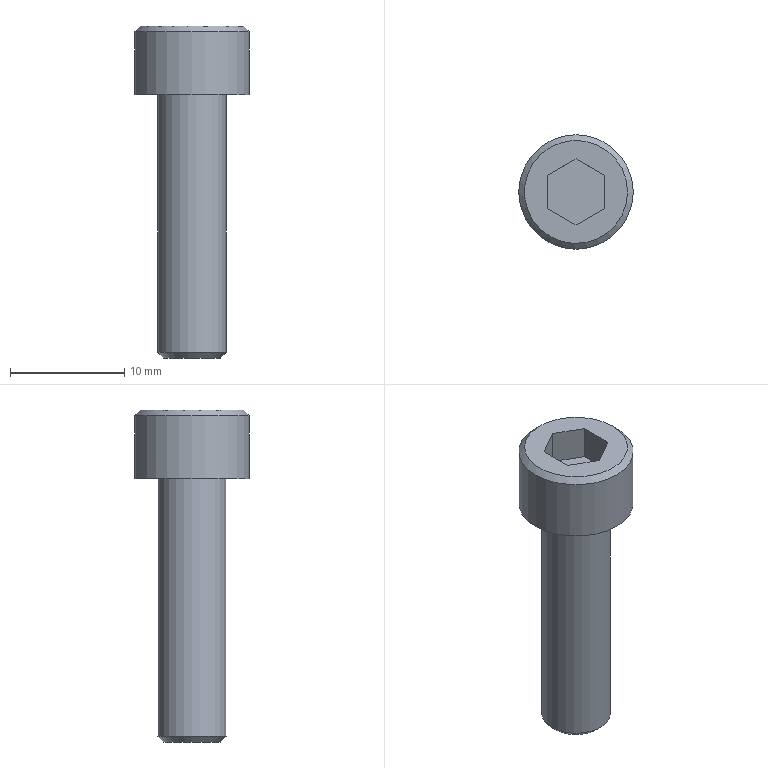Part | STEP file | M6.00-20.00_id118_x_t | 1 solid | 14 faces | box 10 x 10 x 29 mm | volume 1051 mm3 | plane 10 | cylinder 2 | cone 2 | commonest cylinder face diameters 6 x1 10 x1
STEP:
#1=CARTESIAN_POINT('',(-35.5,-80.,-101.5));
#2=VERTEX_POINT('',#1);
#3=CARTESIAN_POINT('',(-40.,-80.,-101.5));
#4=DIRECTION('',(0.,0.,1.));
#5=DIRECTION('',(1.,0.,0.));
#6=AXIS2_PLACEMENT_3D('',#3,#4,#5);
#7=CIRCLE('',#6,4.5);
#8=EDGE_CURVE('',#2,#2,#7,.T.);
#9=ORIENTED_EDGE('',*,*,#8,.T.);
#10=EDGE_LOOP('',(#9));
#11=FACE_BOUND('',#10,.T.);
#12=CARTESIAN_POINT('',(-42.5,-78.557,-101.5));
#13=VERTEX_POINT('',#12);
#14=CARTESIAN_POINT('',(-42.5,-81.443,-101.5));
#15=VERTEX_POINT('',#14);
#16=CARTESIAN_POINT('',(-42.5,-78.557,-101.5));
#17=DIRECTION('',(0.,-1.,0.));
#18=VECTOR('',#17,1.);
#19=LINE('',#16,#18);
#20=EDGE_CURVE('',#13,#15,#19,.T.);
#21=ORIENTED_EDGE('',*,*,#20,.F.);
#22=CARTESIAN_POINT('',(-40.,-77.113,-101.5));
#23=VERTEX_POINT('',#22);
#24=CARTESIAN_POINT('',(-40.,-77.113,-101.5));
#25=DIRECTION('',(-0.866,-0.5,0.));
#26=VECTOR('',#25,1.);
#27=LINE('',#24,#26);
#28=EDGE_CURVE('',#23,#13,#27,.T.);
#29=ORIENTED_EDGE('',*,*,#28,.F.);
#30=CARTESIAN_POINT('',(-37.5,-78.557,-101.5));
#31=VERTEX_POINT('',#30);
#32=CARTESIAN_POINT('',(-37.5,-78.557,-101.5));
#33=DIRECTION('',(-0.866,0.5,0.));
#34=VECTOR('',#33,1.);
#35=LINE('',#32,#34);
#36=EDGE_CURVE('',#31,#23,#35,.T.);
#37=ORIENTED_EDGE('',*,*,#36,.F.);
#38=CARTESIAN_POINT('',(-37.5,-81.443,-101.5));
#39=VERTEX_POINT('',#38);
#40=CARTESIAN_POINT('',(-37.5,-81.443,-101.5));
#41=DIRECTION('',(0.,1.,0.));
#42=VECTOR('',#41,1.);
#43=LINE('',#40,#42);
#44=EDGE_CURVE('',#39,#31,#43,.T.);
#45=ORIENTED_EDGE('',*,*,#44,.F.);
#46=CARTESIAN_POINT('',(-40.,-82.887,-101.5));
#47=VERTEX_POINT('',#46);
#48=CARTESIAN_POINT('',(-40.,-82.887,-101.5));
#49=DIRECTION('',(0.866,0.5,0.));
#50=VECTOR('',#49,1.);
#51=LINE('',#48,#50);
#52=EDGE_CURVE('',#47,#39,#51,.T.);
#53=ORIENTED_EDGE('',*,*,#52,.F.);
#54=CARTESIAN_POINT('',(-42.5,-81.443,-101.5));
#55=DIRECTION('',(0.866,-0.5,0.));
#56=VECTOR('',#55,1.);
#57=LINE('',#54,#56);
#58=EDGE_CURVE('',#15,#47,#57,.T.);
#59=ORIENTED_EDGE('',*,*,#58,.F.);
#60=EDGE_LOOP('',(#21,#29,#37,#45,#53,#59));
#61=FACE_BOUND('',#60,.T.);
#62=CARTESIAN_POINT('',(-40.,-80.,-101.5));
#63=DIRECTION('',(0.,0.,1.));
#64=DIRECTION('',(1.,0.,0.));
#65=AXIS2_PLACEMENT_3D('',#62,#63,#64);
#66=PLANE('',#65);
#67=ADVANCED_FACE('',(#11,#61),#66,.T.);
#68=CARTESIAN_POINT('',(-43.,-80.,-107.5));
#69=VERTEX_POINT('',#68);
#70=CARTESIAN_POINT('',(-40.,-80.,-107.5));
#71=DIRECTION('',(0.,0.,-1.));
#72=DIRECTION('',(-1.,0.,0.));
#73=AXIS2_PLACEMENT_3D('',#70,#71,#72);
#74=CIRCLE('',#73,3.);
#75=EDGE_CURVE('',#69,#69,#74,.T.);
#76=ORIENTED_EDGE('',*,*,#75,.F.);
#77=EDGE_LOOP('',(#76));
#78=FACE_BOUND('',#77,.T.);
#79=CARTESIAN_POINT('',(-35.,-80.,-107.5));
#80=VERTEX_POINT('',#79);
#81=CARTESIAN_POINT('',(-40.,-80.,-107.5));
#82=DIRECTION('',(0.,0.,1.));
#83=DIRECTION('',(1.,0.,0.));
#84=AXIS2_PLACEMENT_3D('',#81,#82,#83);
#85=CIRCLE('',#84,5.);
#86=EDGE_CURVE('',#80,#80,#85,.T.);
#87=ORIENTED_EDGE('',*,*,#86,.F.);
#88=EDGE_LOOP('',(#87));
#89=FACE_BOUND('',#88,.T.);
#90=CARTESIAN_POINT('',(-40.,-80.,-107.5));
#91=DIRECTION('',(0.,0.,-1.));
#92=DIRECTION('',(-1.,0.,0.));
#93=AXIS2_PLACEMENT_3D('',#90,#91,#92);
#94=PLANE('',#93);
#95=ADVANCED_FACE('',(#78,#89),#94,.T.);
#96=CARTESIAN_POINT('',(-35.,-80.,-102.));
#97=VERTEX_POINT('',#96);
#98=CARTESIAN_POINT('',(-40.,-80.,-102.));
#99=DIRECTION('',(0.,0.,-1.));
#100=DIRECTION('',(1.,0.,0.));
#101=AXIS2_PLACEMENT_3D('',#98,#99,#100);
#102=CIRCLE('',#101,5.);
#103=EDGE_CURVE('',#97,#97,#102,.T.);
#104=ORIENTED_EDGE('',*,*,#103,.T.);
#105=EDGE_LOOP('',(#104));
#106=FACE_BOUND('',#105,.T.);
#107=ORIENTED_EDGE('',*,*,#86,.T.);
#108=EDGE_LOOP('',(#107));
#109=FACE_BOUND('',#108,.T.);
#110=CARTESIAN_POINT('',(-40.,-80.,-107.5));
#111=DIRECTION('',(0.,0.,1.));
#112=DIRECTION('',(1.,0.,0.));
#113=AXIS2_PLACEMENT_3D('',#110,#111,#112);
#114=CYLINDRICAL_SURFACE('',#113,5.);
#115=ADVANCED_FACE('',(#106,#109),#114,.T.);
#116=CARTESIAN_POINT('',(-42.5,-80.,-130.5));
#117=VERTEX_POINT('',#116);
#118=CARTESIAN_POINT('',(-40.,-80.,-130.5));
#119=DIRECTION('',(0.,0.,-1.));
#120=DIRECTION('',(-1.,0.,0.));
#121=AXIS2_PLACEMENT_3D('',#118,#119,#120);
#122=CIRCLE('',#121,2.5);
#123=EDGE_CURVE('',#117,#117,#122,.T.);
#124=ORIENTED_EDGE('',*,*,#123,.T.);
#125=EDGE_LOOP('',(#124));
#126=FACE_OUTER_BOUND('',#125,.T.);
#127=CARTESIAN_POINT('',(-40.,-80.,-130.5));
#128=DIRECTION('',(0.,0.,-1.));
#129=DIRECTION('',(-1.,0.,0.));
#130=AXIS2_PLACEMENT_3D('',#127,#128,#129);
#131=PLANE('',#130);
#132=ADVANCED_FACE('',(#126),#131,.T.);
#133=CARTESIAN_POINT('',(-43.,-80.,-130.));
#134=VERTEX_POINT('',#133);
#135=CARTESIAN_POINT('',(-40.,-80.,-130.));
#136=DIRECTION('',(0.,0.,1.));
#137=DIRECTION('',(-1.,0.,0.));
#138=AXIS2_PLACEMENT_3D('',#135,#136,#137);
#139=CIRCLE('',#138,3.);
#140=EDGE_CURVE('',#134,#134,#139,.T.);
#141=ORIENTED_EDGE('',*,*,#140,.T.);
#142=EDGE_LOOP('',(#141));
#143=FACE_BOUND('',#142,.T.);
#144=ORIENTED_EDGE('',*,*,#75,.T.);
#145=EDGE_LOOP('',(#144));
#146=FACE_BOUND('',#145,.T.);
#147=CARTESIAN_POINT('',(-40.,-80.,-107.5));
#148=DIRECTION('',(0.,0.,-1.));
#149=DIRECTION('',(-1.,0.,0.));
#150=AXIS2_PLACEMENT_3D('',#147,#148,#149);
#151=CYLINDRICAL_SURFACE('',#150,3.);
#152=ADVANCED_FACE('',(#143,#146),#151,.T.);
#153=ORIENTED_EDGE('',*,*,#58,.T.);
#154=CARTESIAN_POINT('',(-40.,-82.887,-104.5));
#155=VERTEX_POINT('',#154);
#156=CARTESIAN_POINT('',(-40.,-82.887,-104.5));
#157=DIRECTION('',(0.,0.,1.));
#158=VECTOR('',#157,1.);
#159=LINE('',#156,#158);
#160=EDGE_CURVE('',#155,#47,#159,.T.);
#161=ORIENTED_EDGE('',*,*,#160,.F.);
#162=CARTESIAN_POINT('',(-42.5,-81.443,-104.5));
#163=VERTEX_POINT('',#162);
#164=CARTESIAN_POINT('',(-42.5,-81.443,-104.5));
#165=DIRECTION('',(0.866,-0.5,0.));
#166=VECTOR('',#165,1.);
#167=LINE('',#164,#166);
#168=EDGE_CURVE('',#163,#155,#167,.T.);
#169=ORIENTED_EDGE('',*,*,#168,.F.);
#170=CARTESIAN_POINT('',(-42.5,-81.443,-104.5));
#171=DIRECTION('',(0.,0.,1.));
#172=VECTOR('',#171,1.);
#173=LINE('',#170,#172);
#174=EDGE_CURVE('',#163,#15,#173,.T.);
#175=ORIENTED_EDGE('',*,*,#174,.T.);
#176=EDGE_LOOP('',(#153,#161,#169,#175));
#177=FACE_OUTER_BOUND('',#176,.T.);
#178=CARTESIAN_POINT('',(-41.25,-82.165,-103.));
#179=DIRECTION('',(-0.5,-0.866,0.));
#180=DIRECTION('',(0.866,-0.5,0.));
#181=AXIS2_PLACEMENT_3D('',#178,#179,#180);
#182=PLANE('',#181);
#183=ADVANCED_FACE('',(#177),#182,.F.);
#184=ORIENTED_EDGE('',*,*,#20,.T.);
#185=ORIENTED_EDGE('',*,*,#174,.F.);
#186=CARTESIAN_POINT('',(-42.5,-78.557,-104.5));
#187=VERTEX_POINT('',#186);
#188=CARTESIAN_POINT('',(-42.5,-78.557,-104.5));
#189=DIRECTION('',(0.,-1.,0.));
#190=VECTOR('',#189,1.);
#191=LINE('',#188,#190);
#192=EDGE_CURVE('',#187,#163,#191,.T.);
#193=ORIENTED_EDGE('',*,*,#192,.F.);
#194=CARTESIAN_POINT('',(-42.5,-78.557,-104.5));
#195=DIRECTION('',(0.,0.,1.));
#196=VECTOR('',#195,1.);
#197=LINE('',#194,#196);
#198=EDGE_CURVE('',#187,#13,#197,.T.);
#199=ORIENTED_EDGE('',*,*,#198,.T.);
#200=EDGE_LOOP('',(#184,#185,#193,#199));
#201=FACE_OUTER_BOUND('',#200,.T.);
#202=CARTESIAN_POINT('',(-42.5,-80.,-103.));
#203=DIRECTION('',(-1.,0.,0.));
#204=DIRECTION('',(0.,0.,1.));
#205=AXIS2_PLACEMENT_3D('',#202,#203,#204);
#206=PLANE('',#205);
#207=ADVANCED_FACE('',(#201),#206,.F.);
#208=ORIENTED_EDGE('',*,*,#28,.T.);
#209=ORIENTED_EDGE('',*,*,#198,.F.);
#210=CARTESIAN_POINT('',(-40.,-77.113,-104.5));
#211=VERTEX_POINT('',#210);
#212=CARTESIAN_POINT('',(-40.,-77.113,-104.5));
#213=DIRECTION('',(-0.866,-0.5,0.));
#214=VECTOR('',#213,1.);
#215=LINE('',#212,#214);
#216=EDGE_CURVE('',#211,#187,#215,.T.);
#217=ORIENTED_EDGE('',*,*,#216,.F.);
#218=CARTESIAN_POINT('',(-40.,-77.113,-104.5));
#219=DIRECTION('',(0.,0.,1.));
#220=VECTOR('',#219,1.);
#221=LINE('',#218,#220);
#222=EDGE_CURVE('',#211,#23,#221,.T.);
#223=ORIENTED_EDGE('',*,*,#222,.T.);
#224=EDGE_LOOP('',(#208,#209,#217,#223));
#225=FACE_OUTER_BOUND('',#224,.T.);
#226=CARTESIAN_POINT('',(-41.25,-77.835,-103.));
#227=DIRECTION('',(-0.5,0.866,0.));
#228=DIRECTION('',(-0.866,-0.5,0.));
#229=AXIS2_PLACEMENT_3D('',#226,#227,#228);
#230=PLANE('',#229);
#231=ADVANCED_FACE('',(#225),#230,.F.);
#232=ORIENTED_EDGE('',*,*,#36,.T.);
#233=ORIENTED_EDGE('',*,*,#222,.F.);
#234=CARTESIAN_POINT('',(-37.5,-78.557,-104.5));
#235=VERTEX_POINT('',#234);
#236=CARTESIAN_POINT('',(-37.5,-78.557,-104.5));
#237=DIRECTION('',(-0.866,0.5,0.));
#238=VECTOR('',#237,1.);
#239=LINE('',#236,#238);
#240=EDGE_CURVE('',#235,#211,#239,.T.);
#241=ORIENTED_EDGE('',*,*,#240,.F.);
#242=CARTESIAN_POINT('',(-37.5,-78.557,-104.5));
#243=DIRECTION('',(0.,0.,1.));
#244=VECTOR('',#243,1.);
#245=LINE('',#242,#244);
#246=EDGE_CURVE('',#235,#31,#245,.T.);
#247=ORIENTED_EDGE('',*,*,#246,.T.);
#248=EDGE_LOOP('',(#232,#233,#241,#247));
#249=FACE_OUTER_BOUND('',#248,.T.);
#250=CARTESIAN_POINT('',(-38.75,-77.835,-103.));
#251=DIRECTION('',(0.5,0.866,0.));
#252=DIRECTION('',(-0.866,0.5,0.));
#253=AXIS2_PLACEMENT_3D('',#250,#251,#252);
#254=PLANE('',#253);
#255=ADVANCED_FACE('',(#249),#254,.F.);
#256=ORIENTED_EDGE('',*,*,#44,.T.);
#257=ORIENTED_EDGE('',*,*,#246,.F.);
#258=CARTESIAN_POINT('',(-37.5,-81.443,-104.5));
#259=VERTEX_POINT('',#258);
#260=CARTESIAN_POINT('',(-37.5,-81.443,-104.5));
#261=DIRECTION('',(0.,1.,0.));
#262=VECTOR('',#261,1.);
#263=LINE('',#260,#262);
#264=EDGE_CURVE('',#259,#235,#263,.T.);
#265=ORIENTED_EDGE('',*,*,#264,.F.);
#266=CARTESIAN_POINT('',(-37.5,-81.443,-104.5));
#267=DIRECTION('',(0.,0.,1.));
#268=VECTOR('',#267,1.);
#269=LINE('',#266,#268);
#270=EDGE_CURVE('',#259,#39,#269,.T.);
#271=ORIENTED_EDGE('',*,*,#270,.T.);
#272=EDGE_LOOP('',(#256,#257,#265,#271));
#273=FACE_OUTER_BOUND('',#272,.T.);
#274=CARTESIAN_POINT('',(-37.5,-80.,-103.));
#275=DIRECTION('',(1.,0.,0.));
#276=DIRECTION('',(0.,0.,-1.));
#277=AXIS2_PLACEMENT_3D('',#274,#275,#276);
#278=PLANE('',#277);
#279=ADVANCED_FACE('',(#273),#278,.F.);
#280=ORIENTED_EDGE('',*,*,#52,.T.);
#281=ORIENTED_EDGE('',*,*,#270,.F.);
#282=CARTESIAN_POINT('',(-40.,-82.887,-104.5));
#283=DIRECTION('',(0.866,0.5,0.));
#284=VECTOR('',#283,1.);
#285=LINE('',#282,#284);
#286=EDGE_CURVE('',#155,#259,#285,.T.);
#287=ORIENTED_EDGE('',*,*,#286,.F.);
#288=ORIENTED_EDGE('',*,*,#160,.T.);
#289=EDGE_LOOP('',(#280,#281,#287,#288));
#290=FACE_OUTER_BOUND('',#289,.T.);
#291=CARTESIAN_POINT('',(-38.75,-82.165,-103.));
#292=DIRECTION('',(0.5,-0.866,0.));
#293=DIRECTION('',(0.866,0.5,0.));
#294=AXIS2_PLACEMENT_3D('',#291,#292,#293);
#295=PLANE('',#294);
#296=ADVANCED_FACE('',(#290),#295,.F.);
#297=ORIENTED_EDGE('',*,*,#286,.T.);
#298=ORIENTED_EDGE('',*,*,#264,.T.);
#299=ORIENTED_EDGE('',*,*,#240,.T.);
#300=ORIENTED_EDGE('',*,*,#216,.T.);
#301=ORIENTED_EDGE('',*,*,#192,.T.);
#302=ORIENTED_EDGE('',*,*,#168,.T.);
#303=EDGE_LOOP('',(#297,#298,#299,#300,#301,#302));
#304=FACE_OUTER_BOUND('',#303,.T.);
#305=CARTESIAN_POINT('',(-40.,-80.,-104.5));
#306=DIRECTION('',(0.,0.,-1.));
#307=DIRECTION('',(-1.,0.,0.));
#308=AXIS2_PLACEMENT_3D('',#305,#306,#307);
#309=PLANE('',#308);
#310=ADVANCED_FACE('',(#304),#309,.F.);
#311=ORIENTED_EDGE('',*,*,#123,.F.);
#312=EDGE_LOOP('',(#311));
#313=FACE_BOUND('',#312,.T.);
#314=ORIENTED_EDGE('',*,*,#140,.F.);
#315=EDGE_LOOP('',(#314));
#316=FACE_BOUND('',#315,.T.);
#317=CARTESIAN_POINT('',(-40.,-80.,-130.));
#318=DIRECTION('',(0.,0.,1.));
#319=DIRECTION('',(1.,0.,0.));
#320=AXIS2_PLACEMENT_3D('',#317,#318,#319);
#321=CONICAL_SURFACE('',#320,3.,45.);
#322=ADVANCED_FACE('',(#313,#316),#321,.T.);
#323=ORIENTED_EDGE('',*,*,#8,.F.);
#324=EDGE_LOOP('',(#323));
#325=FACE_BOUND('',#324,.T.);
#326=ORIENTED_EDGE('',*,*,#103,.F.);
#327=EDGE_LOOP('',(#326));
#328=FACE_BOUND('',#327,.T.);
#329=CARTESIAN_POINT('',(-40.,-80.,-102.));
#330=DIRECTION('',(0.,0.,-1.));
#331=DIRECTION('',(-1.,0.,0.));
#332=AXIS2_PLACEMENT_3D('',#329,#330,#331);
#333=CONICAL_SURFACE('',#332,5.,45.);
#334=ADVANCED_FACE('',(#325,#328),#333,.T.);
#335=CLOSED_SHELL('',(#67,#95,#115,#132,#152,#183,#207,#231,#255,#279,#296,#310,#322,#334));
#336=MANIFOLD_SOLID_BREP('',#335);
#337=(LENGTH_UNIT()NAMED_UNIT(*)SI_UNIT(.MILLI.,.METRE.));
#338=UNCERTAINTY_MEASURE_WITH_UNIT(LENGTH_MEASURE(0.00002),#337,'','');
#339=(NAMED_UNIT(*)PLANE_ANGLE_UNIT()SI_UNIT($,.RADIAN.));
#340=PLANE_ANGLE_MEASURE_WITH_UNIT(PLANE_ANGLE_MEASURE(0.01745),#339);
#341=DIMENSIONAL_EXPONENTS(0.,0.,0.,0.,0.,0.,0.);
#342=(CONVERSION_BASED_UNIT('DEGREE',#340)NAMED_UNIT(#341)PLANE_ANGLE_UNIT());
#343=(NAMED_UNIT(*)SI_UNIT($,.STERADIAN.)SOLID_ANGLE_UNIT());
#344=(GEOMETRIC_REPRESENTATION_CONTEXT(3)GLOBAL_UNCERTAINTY_ASSIGNED_CONTEXT((#338))GLOBAL_UNIT_ASSIGNED_CONTEXT((#337,#342,#343))REPRESENTATION_CONTEXT('',''));
#345=ADVANCED_BREP_SHAPE_REPRESENTATION('',(#336),#344);